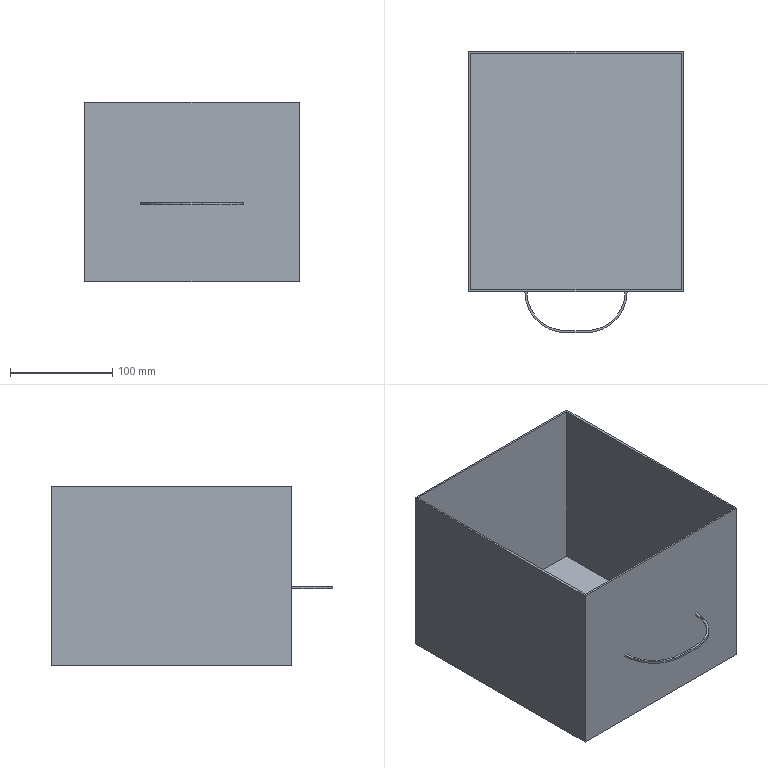Part | NX | features solid 2 | 1 solid | 19 faces | box 210 x 275 x 175 mm | volume 404442 mm3 | plane 15 | cylinder 4 | commonest cylinder face diameters 76 x2 80 x2
STEP:
#1=CARTESIAN_POINT('',(-105.,-535.,-280.));
#2=VERTEX_POINT('',#1);
#3=CARTESIAN_POINT('',(-105.,-770.,-280.));
#4=VERTEX_POINT('',#3);
#5=CARTESIAN_POINT('',(-105.,-510.,-280.));
#6=DIRECTION('',(0.,-1.,0.));
#7=VECTOR('',#6,1000.);
#8=LINE('',#5,#7);
#9=EDGE_CURVE('',#2,#4,#8,.T.);
#10=ORIENTED_EDGE('',*,*,#9,.F.);
#11=CARTESIAN_POINT('',(-105.,-535.,-455.));
#12=VERTEX_POINT('',#11);
#13=CARTESIAN_POINT('',(-105.,-535.,-455.));
#14=DIRECTION('',(0.,0.,1.));
#15=VECTOR('',#14,1000.);
#16=LINE('',#13,#15);
#17=EDGE_CURVE('',#12,#2,#16,.T.);
#18=ORIENTED_EDGE('',*,*,#17,.F.);
#19=CARTESIAN_POINT('',(-105.,-770.,-455.));
#20=VERTEX_POINT('',#19);
#21=CARTESIAN_POINT('',(-105.,-510.,-455.));
#22=DIRECTION('',(0.,-1.,0.));
#23=VECTOR('',#22,1000.);
#24=LINE('',#21,#23);
#25=EDGE_CURVE('',#12,#20,#24,.T.);
#26=ORIENTED_EDGE('',*,*,#25,.T.);
#27=CARTESIAN_POINT('',(-105.,-770.,-90.));
#28=DIRECTION('',(0.,0.,-1.));
#29=VECTOR('',#28,1000.);
#30=LINE('',#27,#29);
#31=EDGE_CURVE('',#4,#20,#30,.T.);
#32=ORIENTED_EDGE('',*,*,#31,.F.);
#33=EDGE_LOOP('',(#10,#18,#26,#32));
#34=FACE_BOUND('',#33,.T.);
#35=CARTESIAN_POINT('',(-105.,-510.,-455.));
#36=DIRECTION('',(1.,0.,0.));
#37=DIRECTION('',(0.,-1.,0.));
#38=AXIS2_PLACEMENT_3D('',#35,#36,#37);
#39=PLANE('',#38);
#40=ADVANCED_FACE('',(#34),#39,.F.);
#41=CARTESIAN_POINT('',(105.,-770.,-280.));
#42=VERTEX_POINT('',#41);
#43=CARTESIAN_POINT('',(105.,-535.,-280.));
#44=VERTEX_POINT('',#43);
#45=CARTESIAN_POINT('',(105.,-510.,-280.));
#46=DIRECTION('',(0.,-1.,0.));
#47=VECTOR('',#46,1000.);
#48=LINE('',#45,#47);
#49=EDGE_CURVE('',#42,#44,#48,.F.);
#50=ORIENTED_EDGE('',*,*,#49,.F.);
#51=CARTESIAN_POINT('',(105.,-770.,-455.));
#52=VERTEX_POINT('',#51);
#53=CARTESIAN_POINT('',(105.,-770.,-455.));
#54=DIRECTION('',(0.,0.,1.));
#55=VECTOR('',#54,1000.);
#56=LINE('',#53,#55);
#57=EDGE_CURVE('',#42,#52,#56,.F.);
#58=ORIENTED_EDGE('',*,*,#57,.T.);
#59=CARTESIAN_POINT('',(105.,-535.,-455.));
#60=VERTEX_POINT('',#59);
#61=CARTESIAN_POINT('',(105.,-510.,-455.));
#62=DIRECTION('',(0.,1.,0.));
#63=VECTOR('',#62,1000.);
#64=LINE('',#61,#63);
#65=EDGE_CURVE('',#60,#52,#64,.F.);
#66=ORIENTED_EDGE('',*,*,#65,.F.);
#67=CARTESIAN_POINT('',(105.,-535.,-455.));
#68=DIRECTION('',(0.,0.,1.));
#69=VECTOR('',#68,1000.);
#70=LINE('',#67,#69);
#71=EDGE_CURVE('',#44,#60,#70,.F.);
#72=ORIENTED_EDGE('',*,*,#71,.F.);
#73=EDGE_LOOP('',(#50,#58,#66,#72));
#74=FACE_BOUND('',#73,.T.);
#75=CARTESIAN_POINT('',(105.,-510.,-455.));
#76=DIRECTION('',(1.,0.,0.));
#77=DIRECTION('',(0.,-1.,0.));
#78=AXIS2_PLACEMENT_3D('',#75,#76,#77);
#79=PLANE('',#78);
#80=ADVANCED_FACE('',(#74),#79,.T.);
#81=CARTESIAN_POINT('',(48.,-770.,-378.));
#82=VERTEX_POINT('',#81);
#83=CARTESIAN_POINT('',(50.,-770.,-378.));
#84=VERTEX_POINT('',#83);
#85=CARTESIAN_POINT('',(-40.,-770.,-378.));
#86=DIRECTION('',(-1.,0.,0.));
#87=VECTOR('',#86,1000.);
#88=LINE('',#85,#87);
#89=EDGE_CURVE('',#82,#84,#88,.F.);
#90=ORIENTED_EDGE('',*,*,#89,.T.);
#91=CARTESIAN_POINT('',(50.,-770.,-380.));
#92=VERTEX_POINT('',#91);
#93=CARTESIAN_POINT('',(50.,-770.,-380.));
#94=DIRECTION('',(0.,0.,-1.));
#95=VECTOR('',#94,1000.);
#96=LINE('',#93,#95);
#97=EDGE_CURVE('',#84,#92,#96,.T.);
#98=ORIENTED_EDGE('',*,*,#97,.T.);
#99=CARTESIAN_POINT('',(48.,-770.,-380.));
#100=VERTEX_POINT('',#99);
#101=CARTESIAN_POINT('',(-40.,-770.,-380.));
#102=DIRECTION('',(1.,0.,0.));
#103=VECTOR('',#102,1000.);
#104=LINE('',#101,#103);
#105=EDGE_CURVE('',#100,#92,#104,.T.);
#106=ORIENTED_EDGE('',*,*,#105,.F.);
#107=CARTESIAN_POINT('',(48.,-770.,-380.));
#108=DIRECTION('',(0.,0.,1.));
#109=VECTOR('',#108,1000.);
#110=LINE('',#107,#109);
#111=EDGE_CURVE('',#82,#100,#110,.F.);
#112=ORIENTED_EDGE('',*,*,#111,.F.);
#113=EDGE_LOOP('',(#90,#98,#106,#112));
#114=FACE_BOUND('',#113,.T.);
#115=CARTESIAN_POINT('',(-50.,-770.,-380.));
#116=VERTEX_POINT('',#115);
#117=CARTESIAN_POINT('',(-48.,-770.,-380.));
#118=VERTEX_POINT('',#117);
#119=CARTESIAN_POINT('',(-40.,-770.,-380.));
#120=DIRECTION('',(1.,0.,0.));
#121=VECTOR('',#120,1000.);
#122=LINE('',#119,#121);
#123=EDGE_CURVE('',#116,#118,#122,.T.);
#124=ORIENTED_EDGE('',*,*,#123,.F.);
#125=CARTESIAN_POINT('',(-50.,-770.,-378.));
#126=VERTEX_POINT('',#125);
#127=CARTESIAN_POINT('',(-50.,-770.,-380.));
#128=DIRECTION('',(0.,0.,1.));
#129=VECTOR('',#128,1000.);
#130=LINE('',#127,#129);
#131=EDGE_CURVE('',#126,#116,#130,.F.);
#132=ORIENTED_EDGE('',*,*,#131,.F.);
#133=CARTESIAN_POINT('',(-48.,-770.,-378.));
#134=VERTEX_POINT('',#133);
#135=CARTESIAN_POINT('',(-40.,-770.,-378.));
#136=DIRECTION('',(-1.,0.,0.));
#137=VECTOR('',#136,1000.);
#138=LINE('',#135,#137);
#139=EDGE_CURVE('',#126,#134,#138,.F.);
#140=ORIENTED_EDGE('',*,*,#139,.T.);
#141=CARTESIAN_POINT('',(-48.,-770.,-380.));
#142=DIRECTION('',(0.,0.,-1.));
#143=VECTOR('',#142,1000.);
#144=LINE('',#141,#143);
#145=EDGE_CURVE('',#134,#118,#144,.T.);
#146=ORIENTED_EDGE('',*,*,#145,.T.);
#147=EDGE_LOOP('',(#124,#132,#140,#146));
#148=FACE_BOUND('',#147,.T.);
#149=CARTESIAN_POINT('',(-17.,-770.,-280.));
#150=DIRECTION('',(1.,0.,0.));
#151=VECTOR('',#150,1000.);
#152=LINE('',#149,#151);
#153=EDGE_CURVE('',#4,#42,#152,.T.);
#154=ORIENTED_EDGE('',*,*,#153,.F.);
#155=ORIENTED_EDGE('',*,*,#31,.T.);
#156=CARTESIAN_POINT('',(-95.,-770.,-455.));
#157=DIRECTION('',(1.,0.,0.));
#158=VECTOR('',#157,1000.);
#159=LINE('',#156,#158);
#160=EDGE_CURVE('',#20,#52,#159,.T.);
#161=ORIENTED_EDGE('',*,*,#160,.T.);
#162=ORIENTED_EDGE('',*,*,#57,.F.);
#163=EDGE_LOOP('',(#154,#155,#161,#162));
#164=FACE_BOUND('',#163,.T.);
#165=CARTESIAN_POINT('',(-17.,-770.,-90.));
#166=DIRECTION('',(0.,1.,0.));
#167=DIRECTION('',(0.,0.,1.));
#168=AXIS2_PLACEMENT_3D('',#165,#166,#167);
#169=PLANE('',#168);
#170=ADVANCED_FACE('',(#114,#148,#164),#169,.F.);
#171=ORIENTED_EDGE('',*,*,#17,.T.);
#172=CARTESIAN_POINT('',(-125.,-535.,-280.));
#173=DIRECTION('',(1.,0.,0.));
#174=VECTOR('',#173,1000.);
#175=LINE('',#172,#174);
#176=EDGE_CURVE('',#2,#44,#175,.T.);
#177=ORIENTED_EDGE('',*,*,#176,.T.);
#178=ORIENTED_EDGE('',*,*,#71,.T.);
#179=CARTESIAN_POINT('',(-95.,-535.,-455.));
#180=DIRECTION('',(1.,0.,0.));
#181=VECTOR('',#180,1000.);
#182=LINE('',#179,#181);
#183=EDGE_CURVE('',#12,#60,#182,.T.);
#184=ORIENTED_EDGE('',*,*,#183,.F.);
#185=EDGE_LOOP('',(#171,#177,#178,#184));
#186=FACE_BOUND('',#185,.T.);
#187=CARTESIAN_POINT('',(-125.,-535.,-575.));
#188=DIRECTION('',(0.,1.,0.));
#189=DIRECTION('',(0.,0.,1.));
#190=AXIS2_PLACEMENT_3D('',#187,#188,#189);
#191=PLANE('',#190);
#192=ADVANCED_FACE('',(#186),#191,.T.);
#193=ORIENTED_EDGE('',*,*,#25,.F.);
#194=ORIENTED_EDGE('',*,*,#183,.T.);
#195=ORIENTED_EDGE('',*,*,#65,.T.);
#196=ORIENTED_EDGE('',*,*,#160,.F.);
#197=EDGE_LOOP('',(#193,#194,#195,#196));
#198=FACE_BOUND('',#197,.T.);
#199=CARTESIAN_POINT('',(-95.,-510.,-455.));
#200=DIRECTION('',(0.,0.,-1.));
#201=DIRECTION('',(-1.,0.,0.));
#202=AXIS2_PLACEMENT_3D('',#199,#200,#201);
#203=PLANE('',#202);
#204=ADVANCED_FACE('',(#198),#203,.T.);
#205=CARTESIAN_POINT('',(-10.,-808.,-378.));
#206=VERTEX_POINT('',#205);
#207=CARTESIAN_POINT('',(-10.,-770.,-378.));
#208=DIRECTION('',(0.,0.,-1.));
#209=DIRECTION('',(-1.,0.,0.));
#210=AXIS2_PLACEMENT_3D('',#207,#208,#209);
#211=CIRCLE('',#210,38.);
#212=EDGE_CURVE('',#134,#206,#211,.F.);
#213=ORIENTED_EDGE('',*,*,#212,.F.);
#214=ORIENTED_EDGE('',*,*,#139,.F.);
#215=CARTESIAN_POINT('',(-10.,-810.,-378.));
#216=VERTEX_POINT('',#215);
#217=CARTESIAN_POINT('',(-10.,-770.,-378.));
#218=DIRECTION('',(0.,0.,-1.));
#219=DIRECTION('',(-1.,0.,0.));
#220=AXIS2_PLACEMENT_3D('',#217,#218,#219);
#221=CIRCLE('',#220,40.);
#222=EDGE_CURVE('',#126,#216,#221,.F.);
#223=ORIENTED_EDGE('',*,*,#222,.T.);
#224=CARTESIAN_POINT('',(10.,-810.,-378.));
#225=VERTEX_POINT('',#224);
#226=CARTESIAN_POINT('',(-40.,-810.,-378.));
#227=DIRECTION('',(1.,0.,0.));
#228=VECTOR('',#227,1000.);
#229=LINE('',#226,#228);
#230=EDGE_CURVE('',#216,#225,#229,.T.);
#231=ORIENTED_EDGE('',*,*,#230,.T.);
#232=CARTESIAN_POINT('',(10.,-770.,-378.));
#233=DIRECTION('',(0.,0.,-1.));
#234=DIRECTION('',(-1.,0.,0.));
#235=AXIS2_PLACEMENT_3D('',#232,#233,#234);
#236=CIRCLE('',#235,40.);
#237=EDGE_CURVE('',#225,#84,#236,.F.);
#238=ORIENTED_EDGE('',*,*,#237,.T.);
#239=ORIENTED_EDGE('',*,*,#89,.F.);
#240=CARTESIAN_POINT('',(10.,-808.,-378.));
#241=VERTEX_POINT('',#240);
#242=CARTESIAN_POINT('',(10.,-770.,-378.));
#243=DIRECTION('',(0.,0.,-1.));
#244=DIRECTION('',(-1.,0.,0.));
#245=AXIS2_PLACEMENT_3D('',#242,#243,#244);
#246=CIRCLE('',#245,38.);
#247=EDGE_CURVE('',#241,#82,#246,.F.);
#248=ORIENTED_EDGE('',*,*,#247,.F.);
#249=CARTESIAN_POINT('',(-40.,-808.,-378.));
#250=DIRECTION('',(1.,0.,0.));
#251=VECTOR('',#250,1000.);
#252=LINE('',#249,#251);
#253=EDGE_CURVE('',#206,#241,#252,.T.);
#254=ORIENTED_EDGE('',*,*,#253,.F.);
#255=EDGE_LOOP('',(#213,#214,#223,#231,#238,#239,#248,#254));
#256=FACE_BOUND('',#255,.T.);
#257=CARTESIAN_POINT('',(-40.,-770.,-378.));
#258=DIRECTION('',(0.,0.,-1.));
#259=DIRECTION('',(-1.,0.,0.));
#260=AXIS2_PLACEMENT_3D('',#257,#258,#259);
#261=PLANE('',#260);
#262=ADVANCED_FACE('',(#256),#261,.F.);
#263=ORIENTED_EDGE('',*,*,#230,.F.);
#264=CARTESIAN_POINT('',(-10.,-810.,-380.));
#265=VERTEX_POINT('',#264);
#266=CARTESIAN_POINT('',(-10.,-810.,-380.));
#267=DIRECTION('',(0.,0.,-1.));
#268=VECTOR('',#267,1000.);
#269=LINE('',#266,#268);
#270=EDGE_CURVE('',#216,#265,#269,.T.);
#271=ORIENTED_EDGE('',*,*,#270,.T.);
#272=CARTESIAN_POINT('',(10.,-810.,-380.));
#273=VERTEX_POINT('',#272);
#274=CARTESIAN_POINT('',(-40.,-810.,-380.));
#275=DIRECTION('',(1.,0.,0.));
#276=VECTOR('',#275,1000.);
#277=LINE('',#274,#276);
#278=EDGE_CURVE('',#265,#273,#277,.T.);
#279=ORIENTED_EDGE('',*,*,#278,.T.);
#280=CARTESIAN_POINT('',(10.,-810.,-380.));
#281=DIRECTION('',(0.,0.,1.));
#282=VECTOR('',#281,1000.);
#283=LINE('',#280,#282);
#284=EDGE_CURVE('',#273,#225,#283,.T.);
#285=ORIENTED_EDGE('',*,*,#284,.T.);
#286=EDGE_LOOP('',(#263,#271,#279,#285));
#287=FACE_BOUND('',#286,.T.);
#288=CARTESIAN_POINT('',(-40.,-810.,-380.));
#289=DIRECTION('',(0.,1.,0.));
#290=DIRECTION('',(1.,0.,0.));
#291=AXIS2_PLACEMENT_3D('',#288,#289,#290);
#292=PLANE('',#291);
#293=ADVANCED_FACE('',(#287),#292,.F.);
#294=CARTESIAN_POINT('',(-10.,-808.,-380.));
#295=VERTEX_POINT('',#294);
#296=CARTESIAN_POINT('',(-10.,-770.,-380.));
#297=DIRECTION('',(0.,0.,-1.));
#298=DIRECTION('',(-1.,0.,0.));
#299=AXIS2_PLACEMENT_3D('',#296,#297,#298);
#300=CIRCLE('',#299,38.);
#301=EDGE_CURVE('',#295,#118,#300,.T.);
#302=ORIENTED_EDGE('',*,*,#301,.F.);
#303=CARTESIAN_POINT('',(10.,-808.,-380.));
#304=VERTEX_POINT('',#303);
#305=CARTESIAN_POINT('',(-40.,-808.,-380.));
#306=DIRECTION('',(1.,0.,0.));
#307=VECTOR('',#306,1000.);
#308=LINE('',#305,#307);
#309=EDGE_CURVE('',#295,#304,#308,.T.);
#310=ORIENTED_EDGE('',*,*,#309,.T.);
#311=CARTESIAN_POINT('',(10.,-770.,-380.));
#312=DIRECTION('',(0.,0.,-1.));
#313=DIRECTION('',(-1.,0.,0.));
#314=AXIS2_PLACEMENT_3D('',#311,#312,#313);
#315=CIRCLE('',#314,38.);
#316=EDGE_CURVE('',#100,#304,#315,.T.);
#317=ORIENTED_EDGE('',*,*,#316,.F.);
#318=ORIENTED_EDGE('',*,*,#105,.T.);
#319=CARTESIAN_POINT('',(10.,-770.,-380.));
#320=DIRECTION('',(0.,0.,-1.));
#321=DIRECTION('',(-1.,0.,0.));
#322=AXIS2_PLACEMENT_3D('',#319,#320,#321);
#323=CIRCLE('',#322,40.);
#324=EDGE_CURVE('',#92,#273,#323,.T.);
#325=ORIENTED_EDGE('',*,*,#324,.T.);
#326=ORIENTED_EDGE('',*,*,#278,.F.);
#327=CARTESIAN_POINT('',(-10.,-770.,-380.));
#328=DIRECTION('',(0.,0.,-1.));
#329=DIRECTION('',(-1.,0.,0.));
#330=AXIS2_PLACEMENT_3D('',#327,#328,#329);
#331=CIRCLE('',#330,40.);
#332=EDGE_CURVE('',#265,#116,#331,.T.);
#333=ORIENTED_EDGE('',*,*,#332,.T.);
#334=ORIENTED_EDGE('',*,*,#123,.T.);
#335=EDGE_LOOP('',(#302,#310,#317,#318,#325,#326,#333,#334));
#336=FACE_BOUND('',#335,.T.);
#337=CARTESIAN_POINT('',(-40.,-770.,-380.));
#338=DIRECTION('',(0.,0.,-1.));
#339=DIRECTION('',(-1.,0.,0.));
#340=AXIS2_PLACEMENT_3D('',#337,#338,#339);
#341=PLANE('',#340);
#342=ADVANCED_FACE('',(#336),#341,.T.);
#343=ORIENTED_EDGE('',*,*,#222,.F.);
#344=ORIENTED_EDGE('',*,*,#131,.T.);
#345=ORIENTED_EDGE('',*,*,#332,.F.);
#346=ORIENTED_EDGE('',*,*,#270,.F.);
#347=EDGE_LOOP('',(#343,#344,#345,#346));
#348=FACE_BOUND('',#347,.T.);
#349=CARTESIAN_POINT('',(-10.,-770.,-380.));
#350=DIRECTION('',(0.,0.,-1.));
#351=DIRECTION('',(-1.,0.,0.));
#352=AXIS2_PLACEMENT_3D('',#349,#350,#351);
#353=CYLINDRICAL_SURFACE('',#352,40.);
#354=ADVANCED_FACE('',(#348),#353,.T.);
#355=ORIENTED_EDGE('',*,*,#237,.F.);
#356=ORIENTED_EDGE('',*,*,#284,.F.);
#357=ORIENTED_EDGE('',*,*,#324,.F.);
#358=ORIENTED_EDGE('',*,*,#97,.F.);
#359=EDGE_LOOP('',(#355,#356,#357,#358));
#360=FACE_BOUND('',#359,.T.);
#361=CARTESIAN_POINT('',(10.,-770.,-380.));
#362=DIRECTION('',(0.,0.,1.));
#363=DIRECTION('',(1.,0.,0.));
#364=AXIS2_PLACEMENT_3D('',#361,#362,#363);
#365=CYLINDRICAL_SURFACE('',#364,40.);
#366=ADVANCED_FACE('',(#360),#365,.T.);
#367=ORIENTED_EDGE('',*,*,#253,.T.);
#368=CARTESIAN_POINT('',(10.,-808.,-380.));
#369=DIRECTION('',(0.,0.,-1.));
#370=VECTOR('',#369,1000.);
#371=LINE('',#368,#370);
#372=EDGE_CURVE('',#304,#241,#371,.F.);
#373=ORIENTED_EDGE('',*,*,#372,.F.);
#374=ORIENTED_EDGE('',*,*,#309,.F.);
#375=CARTESIAN_POINT('',(-10.,-808.,-380.));
#376=DIRECTION('',(0.,0.,-1.));
#377=VECTOR('',#376,1000.);
#378=LINE('',#375,#377);
#379=EDGE_CURVE('',#206,#295,#378,.T.);
#380=ORIENTED_EDGE('',*,*,#379,.F.);
#381=EDGE_LOOP('',(#367,#373,#374,#380));
#382=FACE_BOUND('',#381,.T.);
#383=CARTESIAN_POINT('',(-40.,-808.,-380.));
#384=DIRECTION('',(0.,1.,0.));
#385=DIRECTION('',(1.,0.,0.));
#386=AXIS2_PLACEMENT_3D('',#383,#384,#385);
#387=PLANE('',#386);
#388=ADVANCED_FACE('',(#382),#387,.T.);
#389=ORIENTED_EDGE('',*,*,#212,.T.);
#390=ORIENTED_EDGE('',*,*,#379,.T.);
#391=ORIENTED_EDGE('',*,*,#301,.T.);
#392=ORIENTED_EDGE('',*,*,#145,.F.);
#393=EDGE_LOOP('',(#389,#390,#391,#392));
#394=FACE_BOUND('',#393,.T.);
#395=CARTESIAN_POINT('',(-10.,-770.,-380.));
#396=DIRECTION('',(0.,0.,-1.));
#397=DIRECTION('',(-1.,0.,0.));
#398=AXIS2_PLACEMENT_3D('',#395,#396,#397);
#399=CYLINDRICAL_SURFACE('',#398,38.);
#400=ADVANCED_FACE('',(#394),#399,.F.);
#401=ORIENTED_EDGE('',*,*,#247,.T.);
#402=ORIENTED_EDGE('',*,*,#111,.T.);
#403=ORIENTED_EDGE('',*,*,#316,.T.);
#404=ORIENTED_EDGE('',*,*,#372,.T.);
#405=EDGE_LOOP('',(#401,#402,#403,#404));
#406=FACE_BOUND('',#405,.T.);
#407=CARTESIAN_POINT('',(10.,-770.,-380.));
#408=DIRECTION('',(0.,0.,1.));
#409=DIRECTION('',(1.,0.,0.));
#410=AXIS2_PLACEMENT_3D('',#407,#408,#409);
#411=CYLINDRICAL_SURFACE('',#410,38.);
#412=ADVANCED_FACE('',(#406),#411,.F.);
#413=CARTESIAN_POINT('',(-103.,-768.,-280.));
#414=VERTEX_POINT('',#413);
#415=CARTESIAN_POINT('',(103.,-768.,-280.));
#416=VERTEX_POINT('',#415);
#417=CARTESIAN_POINT('',(-17.,-768.,-280.));
#418=DIRECTION('',(1.,0.,0.));
#419=VECTOR('',#418,1000.);
#420=LINE('',#417,#419);
#421=EDGE_CURVE('',#414,#416,#420,.T.);
#422=ORIENTED_EDGE('',*,*,#421,.F.);
#423=CARTESIAN_POINT('',(-103.,-537.,-280.));
#424=VERTEX_POINT('',#423);
#425=CARTESIAN_POINT('',(-103.,-510.,-280.));
#426=DIRECTION('',(0.,-1.,0.));
#427=VECTOR('',#426,1000.);
#428=LINE('',#425,#427);
#429=EDGE_CURVE('',#424,#414,#428,.T.);
#430=ORIENTED_EDGE('',*,*,#429,.F.);
#431=CARTESIAN_POINT('',(103.,-537.,-280.));
#432=VERTEX_POINT('',#431);
#433=CARTESIAN_POINT('',(-125.,-537.,-280.));
#434=DIRECTION('',(1.,0.,0.));
#435=VECTOR('',#434,1000.);
#436=LINE('',#433,#435);
#437=EDGE_CURVE('',#424,#432,#436,.T.);
#438=ORIENTED_EDGE('',*,*,#437,.T.);
#439=CARTESIAN_POINT('',(103.,-510.,-280.));
#440=DIRECTION('',(0.,-1.,0.));
#441=VECTOR('',#440,1000.);
#442=LINE('',#439,#441);
#443=EDGE_CURVE('',#416,#432,#442,.F.);
#444=ORIENTED_EDGE('',*,*,#443,.F.);
#445=EDGE_LOOP('',(#422,#430,#438,#444));
#446=FACE_BOUND('',#445,.T.);
#447=ORIENTED_EDGE('',*,*,#9,.T.);
#448=ORIENTED_EDGE('',*,*,#153,.T.);
#449=ORIENTED_EDGE('',*,*,#49,.T.);
#450=ORIENTED_EDGE('',*,*,#176,.F.);
#451=EDGE_LOOP('',(#447,#448,#449,#450));
#452=FACE_BOUND('',#451,.T.);
#453=CARTESIAN_POINT('',(-275.,-640.,-280.));
#454=DIRECTION('',(0.,0.,1.));
#455=DIRECTION('',(1.,0.,0.));
#456=AXIS2_PLACEMENT_3D('',#453,#454,#455);
#457=PLANE('',#456);
#458=ADVANCED_FACE('',(#446,#452),#457,.T.);
#459=CARTESIAN_POINT('',(-103.,-537.,-453.));
#460=VERTEX_POINT('',#459);
#461=CARTESIAN_POINT('',(-103.,-768.,-453.));
#462=VERTEX_POINT('',#461);
#463=CARTESIAN_POINT('',(-103.,-510.,-453.));
#464=DIRECTION('',(0.,-1.,0.));
#465=VECTOR('',#464,1000.);
#466=LINE('',#463,#465);
#467=EDGE_CURVE('',#460,#462,#466,.T.);
#468=ORIENTED_EDGE('',*,*,#467,.T.);
#469=CARTESIAN_POINT('',(103.,-768.,-453.));
#470=VERTEX_POINT('',#469);
#471=CARTESIAN_POINT('',(-95.,-768.,-453.));
#472=DIRECTION('',(1.,0.,0.));
#473=VECTOR('',#472,1000.);
#474=LINE('',#471,#473);
#475=EDGE_CURVE('',#462,#470,#474,.T.);
#476=ORIENTED_EDGE('',*,*,#475,.T.);
#477=CARTESIAN_POINT('',(103.,-537.,-453.));
#478=VERTEX_POINT('',#477);
#479=CARTESIAN_POINT('',(103.,-510.,-453.));
#480=DIRECTION('',(0.,1.,0.));
#481=VECTOR('',#480,1000.);
#482=LINE('',#479,#481);
#483=EDGE_CURVE('',#478,#470,#482,.F.);
#484=ORIENTED_EDGE('',*,*,#483,.F.);
#485=CARTESIAN_POINT('',(-95.,-537.,-453.));
#486=DIRECTION('',(1.,0.,0.));
#487=VECTOR('',#486,1000.);
#488=LINE('',#485,#487);
#489=EDGE_CURVE('',#460,#478,#488,.T.);
#490=ORIENTED_EDGE('',*,*,#489,.F.);
#491=EDGE_LOOP('',(#468,#476,#484,#490));
#492=FACE_BOUND('',#491,.T.);
#493=CARTESIAN_POINT('',(-95.,-510.,-453.));
#494=DIRECTION('',(0.,0.,-1.));
#495=DIRECTION('',(-1.,0.,0.));
#496=AXIS2_PLACEMENT_3D('',#493,#494,#495);
#497=PLANE('',#496);
#498=ADVANCED_FACE('',(#492),#497,.F.);
#499=ORIENTED_EDGE('',*,*,#437,.F.);
#500=CARTESIAN_POINT('',(-103.,-537.,-455.));
#501=DIRECTION('',(0.,0.,1.));
#502=VECTOR('',#501,1000.);
#503=LINE('',#500,#502);
#504=EDGE_CURVE('',#460,#424,#503,.T.);
#505=ORIENTED_EDGE('',*,*,#504,.F.);
#506=ORIENTED_EDGE('',*,*,#489,.T.);
#507=CARTESIAN_POINT('',(103.,-537.,-455.));
#508=DIRECTION('',(0.,0.,1.));
#509=VECTOR('',#508,1000.);
#510=LINE('',#507,#509);
#511=EDGE_CURVE('',#432,#478,#510,.F.);
#512=ORIENTED_EDGE('',*,*,#511,.F.);
#513=EDGE_LOOP('',(#499,#505,#506,#512));
#514=FACE_BOUND('',#513,.T.);
#515=CARTESIAN_POINT('',(-125.,-537.,-575.));
#516=DIRECTION('',(0.,1.,0.));
#517=DIRECTION('',(0.,0.,1.));
#518=AXIS2_PLACEMENT_3D('',#515,#516,#517);
#519=PLANE('',#518);
#520=ADVANCED_FACE('',(#514),#519,.F.);
#521=CARTESIAN_POINT('',(-103.,-768.,-90.));
#522=DIRECTION('',(0.,0.,-1.));
#523=VECTOR('',#522,1000.);
#524=LINE('',#521,#523);
#525=EDGE_CURVE('',#414,#462,#524,.T.);
#526=ORIENTED_EDGE('',*,*,#525,.F.);
#527=ORIENTED_EDGE('',*,*,#421,.T.);
#528=CARTESIAN_POINT('',(103.,-768.,-455.));
#529=DIRECTION('',(0.,0.,1.));
#530=VECTOR('',#529,1000.);
#531=LINE('',#528,#530);
#532=EDGE_CURVE('',#416,#470,#531,.F.);
#533=ORIENTED_EDGE('',*,*,#532,.T.);
#534=ORIENTED_EDGE('',*,*,#475,.F.);
#535=EDGE_LOOP('',(#526,#527,#533,#534));
#536=FACE_BOUND('',#535,.T.);
#537=CARTESIAN_POINT('',(-17.,-768.,-90.));
#538=DIRECTION('',(0.,1.,0.));
#539=DIRECTION('',(0.,0.,1.));
#540=AXIS2_PLACEMENT_3D('',#537,#538,#539);
#541=PLANE('',#540);
#542=ADVANCED_FACE('',(#536),#541,.T.);
#543=ORIENTED_EDGE('',*,*,#532,.F.);
#544=ORIENTED_EDGE('',*,*,#443,.T.);
#545=ORIENTED_EDGE('',*,*,#511,.T.);
#546=ORIENTED_EDGE('',*,*,#483,.T.);
#547=EDGE_LOOP('',(#543,#544,#545,#546));
#548=FACE_BOUND('',#547,.T.);
#549=CARTESIAN_POINT('',(103.,-510.,-455.));
#550=DIRECTION('',(1.,0.,0.));
#551=DIRECTION('',(0.,-1.,0.));
#552=AXIS2_PLACEMENT_3D('',#549,#550,#551);
#553=PLANE('',#552);
#554=ADVANCED_FACE('',(#548),#553,.F.);
#555=ORIENTED_EDGE('',*,*,#504,.T.);
#556=ORIENTED_EDGE('',*,*,#429,.T.);
#557=ORIENTED_EDGE('',*,*,#525,.T.);
#558=ORIENTED_EDGE('',*,*,#467,.F.);
#559=EDGE_LOOP('',(#555,#556,#557,#558));
#560=FACE_BOUND('',#559,.T.);
#561=CARTESIAN_POINT('',(-103.,-510.,-455.));
#562=DIRECTION('',(1.,0.,0.));
#563=DIRECTION('',(0.,-1.,0.));
#564=AXIS2_PLACEMENT_3D('',#561,#562,#563);
#565=PLANE('',#564);
#566=ADVANCED_FACE('',(#560),#565,.T.);
#567=CLOSED_SHELL('',(#40,#80,#170,#192,#204,#262,#293,#342,#354,#366,#388,#400,#412,#458,#498,#520,#542,#554,#566));
#568=MANIFOLD_SOLID_BREP('',#567);
#569=(LENGTH_UNIT()NAMED_UNIT(*)SI_UNIT(.MILLI.,.METRE.));
#570=UNCERTAINTY_MEASURE_WITH_UNIT(LENGTH_MEASURE(0.00001),#569,'','');
#571=(NAMED_UNIT(*)PLANE_ANGLE_UNIT()SI_UNIT($,.RADIAN.));
#572=(NAMED_UNIT(*)SI_UNIT($,.STERADIAN.)SOLID_ANGLE_UNIT());
#573=(GEOMETRIC_REPRESENTATION_CONTEXT(3)GLOBAL_UNCERTAINTY_ASSIGNED_CONTEXT((#570))GLOBAL_UNIT_ASSIGNED_CONTEXT((#569,#571,#572))REPRESENTATION_CONTEXT('',''));
#574=ADVANCED_BREP_SHAPE_REPRESENTATION('',(#568),#573);